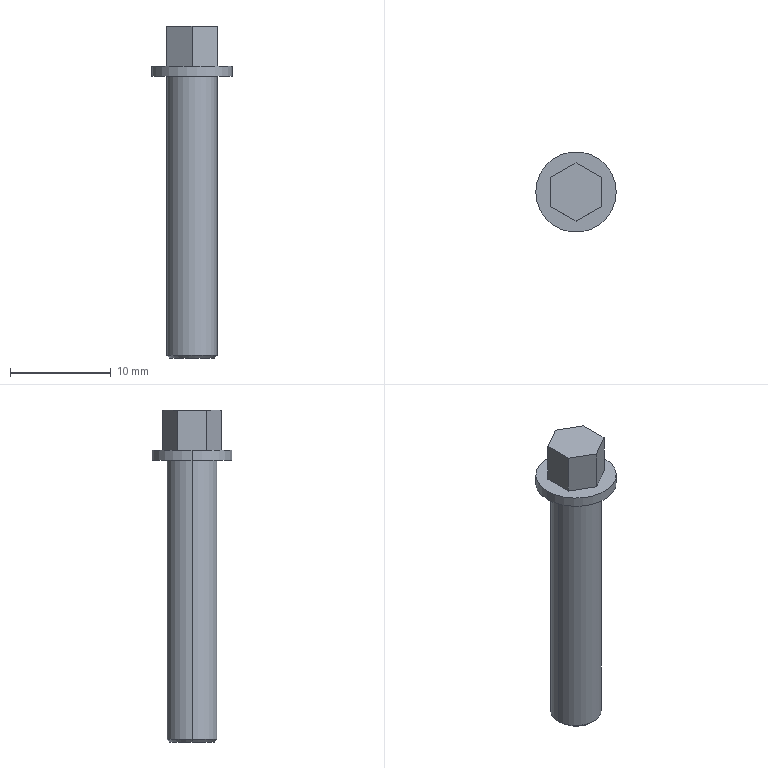Part | SolidWorks | features BaseBody 1 | 1 solid | 16 faces | box 8 x 8 x 33 mm | volume 686.172 mm3 | plane 10 | cylinder 4 | cone 2 | commonest cylinder face diameters 5 x2 8 x2
STEP:
#1=CARTESIAN_POINT('',(2.25,0.,-28.));
#2=VERTEX_POINT('',#1);
#3=CARTESIAN_POINT('',(-2.25,0.,-28.));
#4=VERTEX_POINT('',#3);
#5=CARTESIAN_POINT('',(0.,0.,-28.));
#6=DIRECTION('',(0.,0.,1.));
#7=DIRECTION('',(1.,0.,0.));
#8=AXIS2_PLACEMENT_3D('',#5,#6,#7);
#9=CIRCLE('',#8,2.25);
#10=EDGE_CURVE('',#2,#4,#9,.T.);
#11=ORIENTED_EDGE('',*,*,#10,.T.);
#12=CARTESIAN_POINT('',(-2.5,0.,-27.75));
#13=VERTEX_POINT('',#12);
#14=CARTESIAN_POINT('',(-2.375,0.,-27.875));
#15=DIRECTION('',(-0.7071,0.,0.7071));
#16=VECTOR('',#15,1000.);
#17=LINE('',#14,#16);
#18=EDGE_CURVE('',#4,#13,#17,.T.);
#19=ORIENTED_EDGE('',*,*,#18,.T.);
#20=CARTESIAN_POINT('',(2.5,0.,-27.75));
#21=VERTEX_POINT('',#20);
#22=CARTESIAN_POINT('',(0.,0.,-27.75));
#23=DIRECTION('',(0.,0.,-1.));
#24=DIRECTION('',(1.,0.,0.));
#25=AXIS2_PLACEMENT_3D('',#22,#23,#24);
#26=CIRCLE('',#25,2.5);
#27=EDGE_CURVE('',#13,#21,#26,.T.);
#28=ORIENTED_EDGE('',*,*,#27,.T.);
#29=CARTESIAN_POINT('',(2.375,0.,-27.875));
#30=DIRECTION('',(0.7071,0.,0.7071));
#31=VECTOR('',#30,1000.);
#32=LINE('',#29,#31);
#33=EDGE_CURVE('',#2,#21,#32,.T.);
#34=ORIENTED_EDGE('',*,*,#33,.F.);
#35=EDGE_LOOP('',(#11,#19,#28,#34));
#36=FACE_OUTER_BOUND('',#35,.T.);
#37=CARTESIAN_POINT('',(0.,0.,-27.875));
#38=DIRECTION('',(0.,0.,1.));
#39=DIRECTION('',(1.,0.,0.));
#40=AXIS2_PLACEMENT_3D('',#37,#38,#39);
#41=CONICAL_SURFACE('',#40,2.375,0.7854);
#42=ADVANCED_FACE('',(#36),#41,.T.);
#43=ORIENTED_EDGE('',*,*,#27,.F.);
#44=CARTESIAN_POINT('',(-2.5,0.,0.));
#45=VERTEX_POINT('',#44);
#46=CARTESIAN_POINT('',(-2.5,0.,0.));
#47=DIRECTION('',(0.,0.,1.));
#48=VECTOR('',#47,1000.);
#49=LINE('',#46,#48);
#50=EDGE_CURVE('',#13,#45,#49,.T.);
#51=ORIENTED_EDGE('',*,*,#50,.T.);
#52=CARTESIAN_POINT('',(2.5,0.,0.));
#53=VERTEX_POINT('',#52);
#54=CARTESIAN_POINT('',(0.,0.,0.));
#55=DIRECTION('',(0.,0.,1.));
#56=DIRECTION('',(1.,0.,0.));
#57=AXIS2_PLACEMENT_3D('',#54,#55,#56);
#58=CIRCLE('',#57,2.5);
#59=EDGE_CURVE('',#53,#45,#58,.T.);
#60=ORIENTED_EDGE('',*,*,#59,.F.);
#61=CARTESIAN_POINT('',(2.5,0.,0.));
#62=DIRECTION('',(0.,0.,1.));
#63=VECTOR('',#62,1000.);
#64=LINE('',#61,#63);
#65=EDGE_CURVE('',#21,#53,#64,.T.);
#66=ORIENTED_EDGE('',*,*,#65,.F.);
#67=EDGE_LOOP('',(#43,#51,#60,#66));
#68=FACE_OUTER_BOUND('',#67,.T.);
#69=CARTESIAN_POINT('',(0.,0.,0.));
#70=DIRECTION('',(0.,0.,1.));
#71=DIRECTION('',(1.,0.,0.));
#72=AXIS2_PLACEMENT_3D('',#69,#70,#71);
#73=CYLINDRICAL_SURFACE('',#72,2.5);
#74=ADVANCED_FACE('',(#68),#73,.T.);
#75=CARTESIAN_POINT('',(4.,0.,1.));
#76=VERTEX_POINT('',#75);
#77=CARTESIAN_POINT('',(-4.,0.,1.));
#78=VERTEX_POINT('',#77);
#79=CARTESIAN_POINT('',(0.,0.,1.));
#80=DIRECTION('',(0.,0.,1.));
#81=DIRECTION('',(-1.,0.,0.));
#82=AXIS2_PLACEMENT_3D('',#79,#80,#81);
#83=CIRCLE('',#82,4.);
#84=EDGE_CURVE('',#76,#78,#83,.T.);
#85=ORIENTED_EDGE('',*,*,#84,.F.);
#86=CARTESIAN_POINT('',(4.,0.,0.));
#87=VERTEX_POINT('',#86);
#88=CARTESIAN_POINT('',(4.,0.,0.));
#89=DIRECTION('',(0.,0.,-1.));
#90=VECTOR('',#89,1000.);
#91=LINE('',#88,#90);
#92=EDGE_CURVE('',#76,#87,#91,.T.);
#93=ORIENTED_EDGE('',*,*,#92,.T.);
#94=CARTESIAN_POINT('',(-4.,0.,0.));
#95=VERTEX_POINT('',#94);
#96=CARTESIAN_POINT('',(0.,0.,0.));
#97=DIRECTION('',(0.,0.,-1.));
#98=DIRECTION('',(-1.,0.,0.));
#99=AXIS2_PLACEMENT_3D('',#96,#97,#98);
#100=CIRCLE('',#99,4.);
#101=EDGE_CURVE('',#95,#87,#100,.T.);
#102=ORIENTED_EDGE('',*,*,#101,.F.);
#103=CARTESIAN_POINT('',(-4.,0.,0.));
#104=DIRECTION('',(0.,0.,-1.));
#105=VECTOR('',#104,1000.);
#106=LINE('',#103,#105);
#107=EDGE_CURVE('',#78,#95,#106,.T.);
#108=ORIENTED_EDGE('',*,*,#107,.F.);
#109=EDGE_LOOP('',(#85,#93,#102,#108));
#110=FACE_OUTER_BOUND('',#109,.T.);
#111=CARTESIAN_POINT('',(0.,0.,0.));
#112=DIRECTION('',(0.,0.,-1.));
#113=DIRECTION('',(-1.,0.,0.));
#114=AXIS2_PLACEMENT_3D('',#111,#112,#113);
#115=CYLINDRICAL_SURFACE('',#114,4.);
#116=ADVANCED_FACE('',(#110),#115,.T.);
#117=ORIENTED_EDGE('',*,*,#10,.F.);
#118=CARTESIAN_POINT('',(0.,0.,-28.));
#119=DIRECTION('',(0.,0.,1.));
#120=DIRECTION('',(1.,0.,0.));
#121=AXIS2_PLACEMENT_3D('',#118,#119,#120);
#122=CIRCLE('',#121,2.25);
#123=EDGE_CURVE('',#4,#2,#122,.T.);
#124=ORIENTED_EDGE('',*,*,#123,.F.);
#125=EDGE_LOOP('',(#117,#124));
#126=FACE_OUTER_BOUND('',#125,.T.);
#127=CARTESIAN_POINT('',(0.,0.,-28.));
#128=DIRECTION('',(0.,0.,1.));
#129=DIRECTION('',(1.,0.,0.));
#130=AXIS2_PLACEMENT_3D('',#127,#128,#129);
#131=PLANE('',#130);
#132=ADVANCED_FACE('',(#126),#131,.F.);
#133=CARTESIAN_POINT('',(-2.5,-1.443,1.));
#134=VERTEX_POINT('',#133);
#135=CARTESIAN_POINT('',(-2.5,1.443,1.));
#136=VERTEX_POINT('',#135);
#137=CARTESIAN_POINT('',(-2.5,0.7217,1.));
#138=DIRECTION('',(0.,1.,0.));
#139=VECTOR('',#138,1000.);
#140=LINE('',#137,#139);
#141=EDGE_CURVE('',#134,#136,#140,.T.);
#142=ORIENTED_EDGE('',*,*,#141,.F.);
#143=CARTESIAN_POINT('',(-2.5,-1.443,5.));
#144=VERTEX_POINT('',#143);
#145=CARTESIAN_POINT('',(-2.5,-1.443,1.));
#146=DIRECTION('',(0.,0.,1.));
#147=VECTOR('',#146,1000.);
#148=LINE('',#145,#147);
#149=EDGE_CURVE('',#134,#144,#148,.T.);
#150=ORIENTED_EDGE('',*,*,#149,.T.);
#151=CARTESIAN_POINT('',(-2.5,1.443,5.));
#152=VERTEX_POINT('',#151);
#153=CARTESIAN_POINT('',(-2.5,-1.443,5.));
#154=DIRECTION('',(0.,-1.,0.));
#155=VECTOR('',#154,1000.);
#156=LINE('',#153,#155);
#157=EDGE_CURVE('',#152,#144,#156,.T.);
#158=ORIENTED_EDGE('',*,*,#157,.F.);
#159=CARTESIAN_POINT('',(-2.5,1.443,1.));
#160=DIRECTION('',(0.,0.,1.));
#161=VECTOR('',#160,1000.);
#162=LINE('',#159,#161);
#163=EDGE_CURVE('',#136,#152,#162,.T.);
#164=ORIENTED_EDGE('',*,*,#163,.F.);
#165=EDGE_LOOP('',(#142,#150,#158,#164));
#166=FACE_OUTER_BOUND('',#165,.T.);
#167=CARTESIAN_POINT('',(-2.5,1.443,1.));
#168=DIRECTION('',(-1.,0.,0.));
#169=DIRECTION('',(0.,1.,0.));
#170=AXIS2_PLACEMENT_3D('',#167,#168,#169);
#171=PLANE('',#170);
#172=ADVANCED_FACE('',(#166),#171,.T.);
#173=CARTESIAN_POINT('',(0.,2.887,1.));
#174=VERTEX_POINT('',#173);
#175=CARTESIAN_POINT('',(-0.625,2.526,1.));
#176=DIRECTION('',(0.866,0.5,0.));
#177=VECTOR('',#176,1000.);
#178=LINE('',#175,#177);
#179=EDGE_CURVE('',#136,#174,#178,.T.);
#180=ORIENTED_EDGE('',*,*,#179,.F.);
#181=ORIENTED_EDGE('',*,*,#163,.T.);
#182=CARTESIAN_POINT('',(0.,2.887,5.));
#183=VERTEX_POINT('',#182);
#184=CARTESIAN_POINT('',(-2.5,1.443,5.));
#185=DIRECTION('',(-0.866,-0.5,0.));
#186=VECTOR('',#185,1000.);
#187=LINE('',#184,#186);
#188=EDGE_CURVE('',#183,#152,#187,.T.);
#189=ORIENTED_EDGE('',*,*,#188,.F.);
#190=CARTESIAN_POINT('',(0.,2.887,1.));
#191=DIRECTION('',(0.,0.,1.));
#192=VECTOR('',#191,1000.);
#193=LINE('',#190,#192);
#194=EDGE_CURVE('',#174,#183,#193,.T.);
#195=ORIENTED_EDGE('',*,*,#194,.F.);
#196=EDGE_LOOP('',(#180,#181,#189,#195));
#197=FACE_OUTER_BOUND('',#196,.T.);
#198=CARTESIAN_POINT('',(0.,2.887,1.));
#199=DIRECTION('',(-0.5,0.866,0.));
#200=DIRECTION('',(0.,0.,1.));
#201=AXIS2_PLACEMENT_3D('',#198,#199,#200);
#202=PLANE('',#201);
#203=ADVANCED_FACE('',(#197),#202,.T.);
#204=CARTESIAN_POINT('',(2.5,1.443,1.));
#205=VERTEX_POINT('',#204);
#206=CARTESIAN_POINT('',(1.875,1.804,1.));
#207=DIRECTION('',(0.866,-0.5,0.));
#208=VECTOR('',#207,1000.);
#209=LINE('',#206,#208);
#210=EDGE_CURVE('',#174,#205,#209,.T.);
#211=ORIENTED_EDGE('',*,*,#210,.F.);
#212=ORIENTED_EDGE('',*,*,#194,.T.);
#213=CARTESIAN_POINT('',(2.5,1.443,5.));
#214=VERTEX_POINT('',#213);
#215=CARTESIAN_POINT('',(0.,2.887,5.));
#216=DIRECTION('',(-0.866,0.5,0.));
#217=VECTOR('',#216,1000.);
#218=LINE('',#215,#217);
#219=EDGE_CURVE('',#214,#183,#218,.T.);
#220=ORIENTED_EDGE('',*,*,#219,.F.);
#221=CARTESIAN_POINT('',(2.5,1.443,1.));
#222=DIRECTION('',(0.,0.,1.));
#223=VECTOR('',#222,1000.);
#224=LINE('',#221,#223);
#225=EDGE_CURVE('',#205,#214,#224,.T.);
#226=ORIENTED_EDGE('',*,*,#225,.F.);
#227=EDGE_LOOP('',(#211,#212,#220,#226));
#228=FACE_OUTER_BOUND('',#227,.T.);
#229=CARTESIAN_POINT('',(2.5,1.443,1.));
#230=DIRECTION('',(0.5,0.866,0.));
#231=DIRECTION('',(0.,0.,-1.));
#232=AXIS2_PLACEMENT_3D('',#229,#230,#231);
#233=PLANE('',#232);
#234=ADVANCED_FACE('',(#228),#233,.T.);
#235=CARTESIAN_POINT('',(2.5,-1.443,1.));
#236=VERTEX_POINT('',#235);
#237=CARTESIAN_POINT('',(2.5,-0.7217,1.));
#238=DIRECTION('',(0.,-1.,0.));
#239=VECTOR('',#238,1000.);
#240=LINE('',#237,#239);
#241=EDGE_CURVE('',#205,#236,#240,.T.);
#242=ORIENTED_EDGE('',*,*,#241,.F.);
#243=ORIENTED_EDGE('',*,*,#225,.T.);
#244=CARTESIAN_POINT('',(2.5,-1.443,5.));
#245=VERTEX_POINT('',#244);
#246=CARTESIAN_POINT('',(2.5,1.443,5.));
#247=DIRECTION('',(0.,1.,0.));
#248=VECTOR('',#247,1000.);
#249=LINE('',#246,#248);
#250=EDGE_CURVE('',#245,#214,#249,.T.);
#251=ORIENTED_EDGE('',*,*,#250,.F.);
#252=CARTESIAN_POINT('',(2.5,-1.443,1.));
#253=DIRECTION('',(0.,0.,1.));
#254=VECTOR('',#253,1000.);
#255=LINE('',#252,#254);
#256=EDGE_CURVE('',#236,#245,#255,.T.);
#257=ORIENTED_EDGE('',*,*,#256,.F.);
#258=EDGE_LOOP('',(#242,#243,#251,#257));
#259=FACE_OUTER_BOUND('',#258,.T.);
#260=CARTESIAN_POINT('',(2.5,-1.443,1.));
#261=DIRECTION('',(1.,0.,0.));
#262=DIRECTION('',(0.,-1.,0.));
#263=AXIS2_PLACEMENT_3D('',#260,#261,#262);
#264=PLANE('',#263);
#265=ADVANCED_FACE('',(#259),#264,.T.);
#266=CARTESIAN_POINT('',(0.,-2.887,1.));
#267=VERTEX_POINT('',#266);
#268=CARTESIAN_POINT('',(0.625,-2.526,1.));
#269=DIRECTION('',(-0.866,-0.5,0.));
#270=VECTOR('',#269,1000.);
#271=LINE('',#268,#270);
#272=EDGE_CURVE('',#236,#267,#271,.T.);
#273=ORIENTED_EDGE('',*,*,#272,.F.);
#274=ORIENTED_EDGE('',*,*,#256,.T.);
#275=CARTESIAN_POINT('',(0.,-2.887,5.));
#276=VERTEX_POINT('',#275);
#277=CARTESIAN_POINT('',(2.5,-1.443,5.));
#278=DIRECTION('',(0.866,0.5,0.));
#279=VECTOR('',#278,1000.);
#280=LINE('',#277,#279);
#281=EDGE_CURVE('',#276,#245,#280,.T.);
#282=ORIENTED_EDGE('',*,*,#281,.F.);
#283=CARTESIAN_POINT('',(0.,-2.887,1.));
#284=DIRECTION('',(0.,0.,1.));
#285=VECTOR('',#284,1000.);
#286=LINE('',#283,#285);
#287=EDGE_CURVE('',#267,#276,#286,.T.);
#288=ORIENTED_EDGE('',*,*,#287,.F.);
#289=EDGE_LOOP('',(#273,#274,#282,#288));
#290=FACE_OUTER_BOUND('',#289,.T.);
#291=CARTESIAN_POINT('',(0.,-2.887,1.));
#292=DIRECTION('',(0.5,-0.866,0.));
#293=DIRECTION('',(0.,0.,-1.));
#294=AXIS2_PLACEMENT_3D('',#291,#292,#293);
#295=PLANE('',#294);
#296=ADVANCED_FACE('',(#290),#295,.T.);
#297=CARTESIAN_POINT('',(-1.875,-1.804,1.));
#298=DIRECTION('',(-0.866,0.5,0.));
#299=VECTOR('',#298,1000.);
#300=LINE('',#297,#299);
#301=EDGE_CURVE('',#267,#134,#300,.T.);
#302=ORIENTED_EDGE('',*,*,#301,.F.);
#303=ORIENTED_EDGE('',*,*,#287,.T.);
#304=CARTESIAN_POINT('',(0.,-2.887,5.));
#305=DIRECTION('',(0.866,-0.5,0.));
#306=VECTOR('',#305,1000.);
#307=LINE('',#304,#306);
#308=EDGE_CURVE('',#144,#276,#307,.T.);
#309=ORIENTED_EDGE('',*,*,#308,.F.);
#310=ORIENTED_EDGE('',*,*,#149,.F.);
#311=EDGE_LOOP('',(#302,#303,#309,#310));
#312=FACE_OUTER_BOUND('',#311,.T.);
#313=CARTESIAN_POINT('',(-2.5,-1.443,1.));
#314=DIRECTION('',(-0.5,-0.866,0.));
#315=DIRECTION('',(-0.866,0.5,0.));
#316=AXIS2_PLACEMENT_3D('',#313,#314,#315);
#317=PLANE('',#316);
#318=ADVANCED_FACE('',(#312),#317,.T.);
#319=ORIENTED_EDGE('',*,*,#308,.T.);
#320=ORIENTED_EDGE('',*,*,#281,.T.);
#321=ORIENTED_EDGE('',*,*,#250,.T.);
#322=ORIENTED_EDGE('',*,*,#219,.T.);
#323=ORIENTED_EDGE('',*,*,#188,.T.);
#324=ORIENTED_EDGE('',*,*,#157,.T.);
#325=EDGE_LOOP('',(#319,#320,#321,#322,#323,#324));
#326=FACE_OUTER_BOUND('',#325,.T.);
#327=CARTESIAN_POINT('',(0.,0.,5.));
#328=DIRECTION('',(0.,0.,1.));
#329=DIRECTION('',(1.,0.,0.));
#330=AXIS2_PLACEMENT_3D('',#327,#328,#329);
#331=PLANE('',#330);
#332=ADVANCED_FACE('',(#326),#331,.T.);
#333=ORIENTED_EDGE('',*,*,#59,.T.);
#334=CARTESIAN_POINT('',(0.,0.,0.));
#335=DIRECTION('',(0.,0.,1.));
#336=DIRECTION('',(1.,0.,0.));
#337=AXIS2_PLACEMENT_3D('',#334,#335,#336);
#338=CIRCLE('',#337,2.5);
#339=EDGE_CURVE('',#45,#53,#338,.T.);
#340=ORIENTED_EDGE('',*,*,#339,.T.);
#341=EDGE_LOOP('',(#333,#340));
#342=FACE_BOUND('',#341,.T.);
#343=ORIENTED_EDGE('',*,*,#101,.T.);
#344=CARTESIAN_POINT('',(0.,0.,0.));
#345=DIRECTION('',(0.,0.,-1.));
#346=DIRECTION('',(-1.,0.,0.));
#347=AXIS2_PLACEMENT_3D('',#344,#345,#346);
#348=CIRCLE('',#347,4.);
#349=EDGE_CURVE('',#87,#95,#348,.T.);
#350=ORIENTED_EDGE('',*,*,#349,.T.);
#351=EDGE_LOOP('',(#343,#350));
#352=FACE_OUTER_BOUND('',#351,.T.);
#353=CARTESIAN_POINT('',(0.,0.,0.));
#354=DIRECTION('',(0.,0.,1.));
#355=DIRECTION('',(1.,0.,0.));
#356=AXIS2_PLACEMENT_3D('',#353,#354,#355);
#357=PLANE('',#356);
#358=ADVANCED_FACE('',(#342,#352),#357,.F.);
#359=ORIENTED_EDGE('',*,*,#141,.T.);
#360=ORIENTED_EDGE('',*,*,#179,.T.);
#361=ORIENTED_EDGE('',*,*,#210,.T.);
#362=ORIENTED_EDGE('',*,*,#241,.T.);
#363=ORIENTED_EDGE('',*,*,#272,.T.);
#364=ORIENTED_EDGE('',*,*,#301,.T.);
#365=EDGE_LOOP('',(#359,#360,#361,#362,#363,#364));
#366=FACE_BOUND('',#365,.T.);
#367=CARTESIAN_POINT('',(0.,0.,1.));
#368=DIRECTION('',(0.,0.,1.));
#369=DIRECTION('',(-1.,0.,0.));
#370=AXIS2_PLACEMENT_3D('',#367,#368,#369);
#371=CIRCLE('',#370,4.);
#372=EDGE_CURVE('',#78,#76,#371,.T.);
#373=ORIENTED_EDGE('',*,*,#372,.T.);
#374=ORIENTED_EDGE('',*,*,#84,.T.);
#375=EDGE_LOOP('',(#373,#374));
#376=FACE_OUTER_BOUND('',#375,.T.);
#377=CARTESIAN_POINT('',(0.,0.,1.));
#378=DIRECTION('',(0.,0.,1.));
#379=DIRECTION('',(1.,0.,0.));
#380=AXIS2_PLACEMENT_3D('',#377,#378,#379);
#381=PLANE('',#380);
#382=ADVANCED_FACE('',(#366,#376),#381,.T.);
#383=ORIENTED_EDGE('',*,*,#92,.F.);
#384=ORIENTED_EDGE('',*,*,#372,.F.);
#385=ORIENTED_EDGE('',*,*,#107,.T.);
#386=ORIENTED_EDGE('',*,*,#349,.F.);
#387=EDGE_LOOP('',(#383,#384,#385,#386));
#388=FACE_OUTER_BOUND('',#387,.T.);
#389=CARTESIAN_POINT('',(0.,0.,0.));
#390=DIRECTION('',(0.,0.,-1.));
#391=DIRECTION('',(-1.,0.,0.));
#392=AXIS2_PLACEMENT_3D('',#389,#390,#391);
#393=CYLINDRICAL_SURFACE('',#392,4.);
#394=ADVANCED_FACE('',(#388),#393,.T.);
#395=ORIENTED_EDGE('',*,*,#50,.F.);
#396=CARTESIAN_POINT('',(0.,0.,-27.75));
#397=DIRECTION('',(0.,0.,-1.));
#398=DIRECTION('',(1.,0.,0.));
#399=AXIS2_PLACEMENT_3D('',#396,#397,#398);
#400=CIRCLE('',#399,2.5);
#401=EDGE_CURVE('',#21,#13,#400,.T.);
#402=ORIENTED_EDGE('',*,*,#401,.F.);
#403=ORIENTED_EDGE('',*,*,#65,.T.);
#404=ORIENTED_EDGE('',*,*,#339,.F.);
#405=EDGE_LOOP('',(#395,#402,#403,#404));
#406=FACE_OUTER_BOUND('',#405,.T.);
#407=CARTESIAN_POINT('',(0.,0.,0.));
#408=DIRECTION('',(0.,0.,1.));
#409=DIRECTION('',(1.,0.,0.));
#410=AXIS2_PLACEMENT_3D('',#407,#408,#409);
#411=CYLINDRICAL_SURFACE('',#410,2.5);
#412=ADVANCED_FACE('',(#406),#411,.T.);
#413=ORIENTED_EDGE('',*,*,#18,.F.);
#414=ORIENTED_EDGE('',*,*,#123,.T.);
#415=ORIENTED_EDGE('',*,*,#33,.T.);
#416=ORIENTED_EDGE('',*,*,#401,.T.);
#417=EDGE_LOOP('',(#413,#414,#415,#416));
#418=FACE_OUTER_BOUND('',#417,.T.);
#419=CARTESIAN_POINT('',(0.,0.,-27.875));
#420=DIRECTION('',(0.,0.,1.));
#421=DIRECTION('',(1.,0.,0.));
#422=AXIS2_PLACEMENT_3D('',#419,#420,#421);
#423=CONICAL_SURFACE('',#422,2.375,0.7854);
#424=ADVANCED_FACE('',(#418),#423,.T.);
#425=CLOSED_SHELL('',(#42,#74,#116,#132,#172,#203,#234,#265,#296,#318,#332,#358,#382,#394,#412,#424));
#426=MANIFOLD_SOLID_BREP('',#425);
#427=CARTESIAN_POINT('',(0.,0.,0.));
#428=DIRECTION('',(0.,0.,1.));
#429=DIRECTION('',(1.,0.,0.));
#430=AXIS2_PLACEMENT_3D('',#427,#428,#429);
#431=(LENGTH_UNIT()NAMED_UNIT(*)SI_UNIT(.MILLI.,.METRE.));
#432=UNCERTAINTY_MEASURE_WITH_UNIT(LENGTH_MEASURE(0.00001),#431,'','');
#433=(NAMED_UNIT(*)PLANE_ANGLE_UNIT()SI_UNIT($,.RADIAN.));
#434=(NAMED_UNIT(*)SI_UNIT($,.STERADIAN.)SOLID_ANGLE_UNIT());
#435=(GEOMETRIC_REPRESENTATION_CONTEXT(3)GLOBAL_UNCERTAINTY_ASSIGNED_CONTEXT((#432))GLOBAL_UNIT_ASSIGNED_CONTEXT((#431,#433,#434))REPRESENTATION_CONTEXT('',''));
#436=ADVANCED_BREP_SHAPE_REPRESENTATION('',(#426,#430),#435);